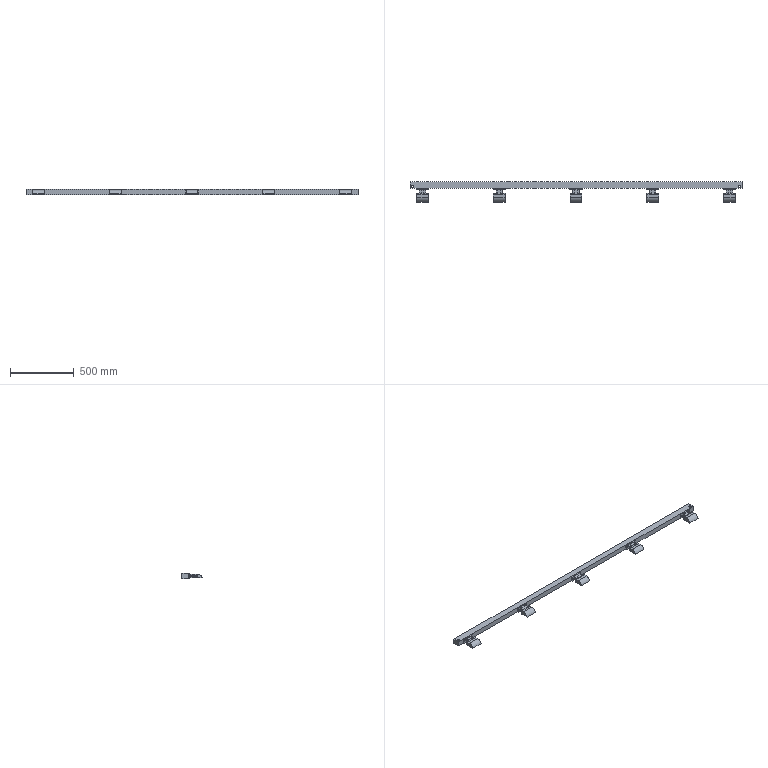Part | SolidWorks | features ReferencePattern 12, CompositeCurve 9, LocalLPattern 1 | 16 solids | 640 faces | box 2596 x 157.44 x 40 mm | volume 6283674 mm3 | cylinder 354 | plane 246 | spline 40 | commonest cylinder face diameters 12 x250 5 x40 10.5 x35 8 x20 76 x5 16 x4